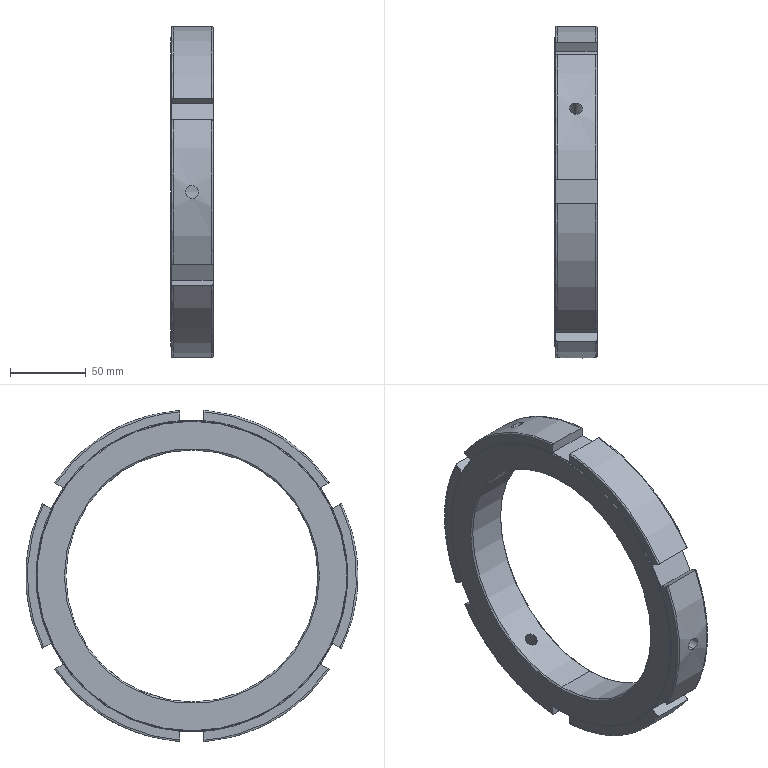Part | SolidWorks | features BaseBody 1 | 1 solid | 60 faces | box 28 x 220 x 219.417 mm | volume 425123 mm3 | plane 26 | spline 14 | cylinder 14 | cone 6 | commonest cylinder face diameters 8.5 x6 220 x6 167 x2